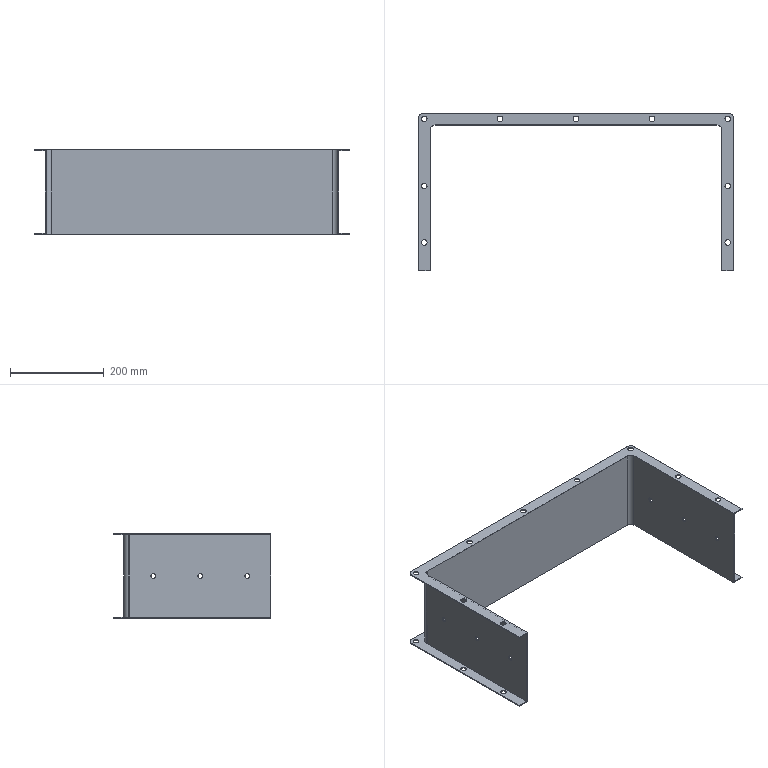Part | SolidWorks | features ICE 3, Cut 1, Extrusion 1 | 1 solid | 74 faces | box 670 x 335 x 180 mm | volume 671550 mm3 | cylinder 56 | plane 18 | commonest cylinder face diameters 12 x36 10 x12 20 x8